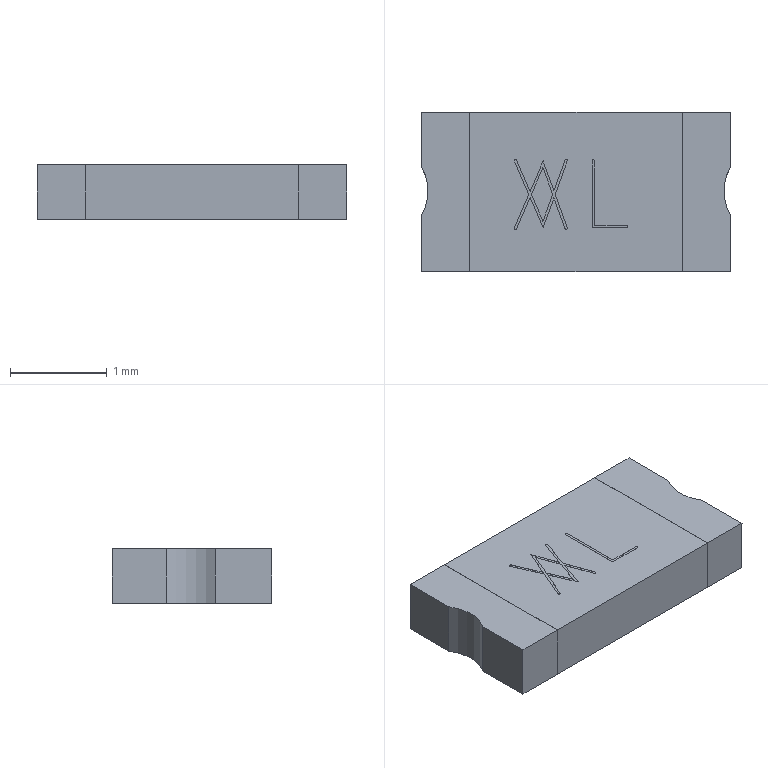Part | STEP file | RJ-USIO-V1_2-220411_3 | 1 solid | 52 faces | box 3.202 x 1.652 x 0.562 mm | volume 2.935 mm3 | plane 41 | cylinder 11 | commonest cylinder face diameters 0.025 x9 0.927 x2